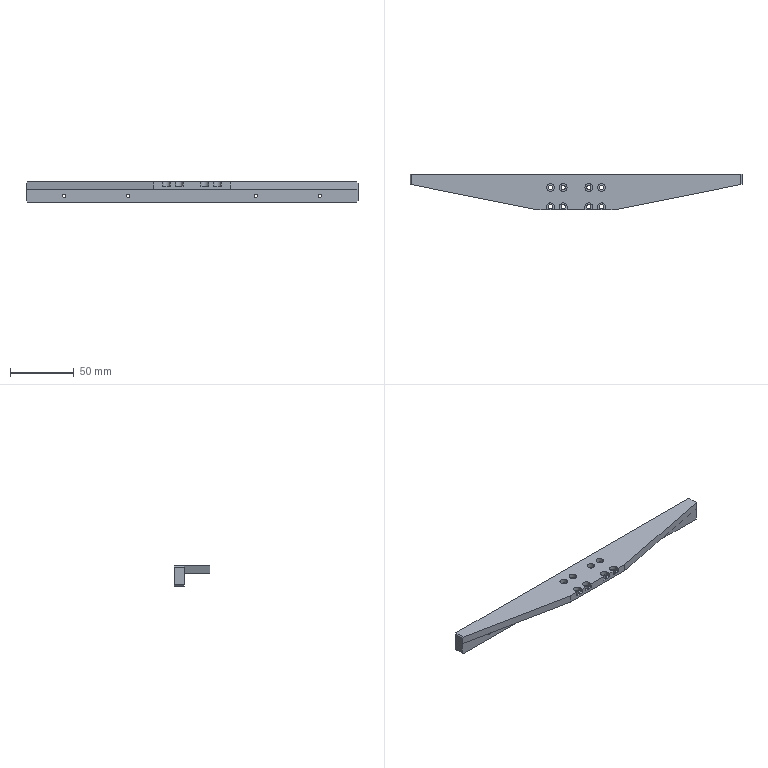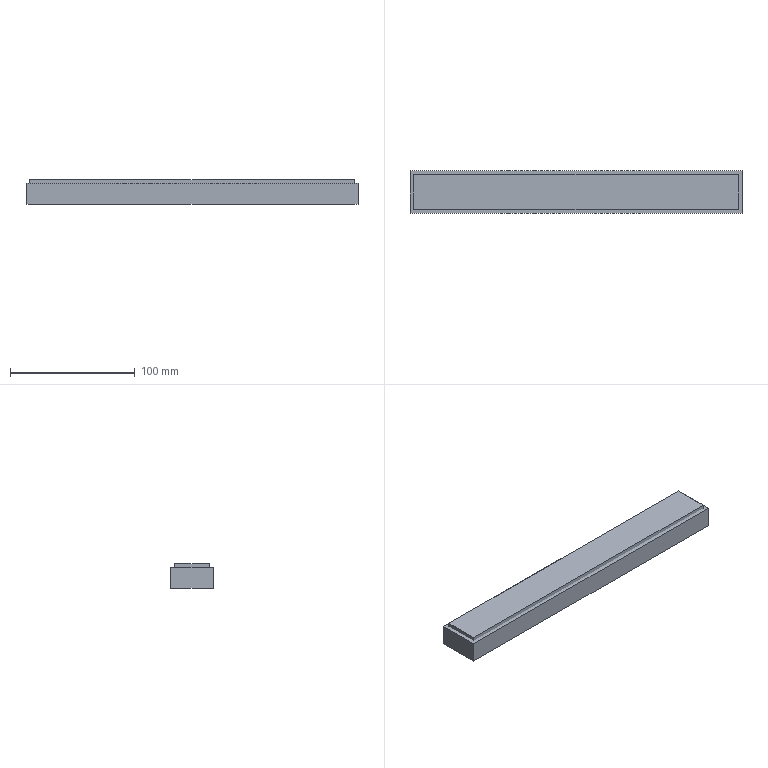CAM job | NX | 3+2 milling, drilling | part box 260 x 28 x 16 mm | stock box 266 x 34 x 20 mm
Tools:
number,name,description,diameter,corner_radius,flute_length,length,flutes
19,D80,Milling Tool-5 Parameters,80.0,0.0,50.0,75.0,2
15,D10,Milling Tool-5 Parameters,10.0,0.0,50.0,75.0,2
14,D10JING,Milling Tool-5 Parameters,10.0,0.0,50.0,75.0,2
1,D6A45,Milling Tool-5 Parameters,6.0,0.0,50.0,75.0,2
16,3.4ZT,Drilling Tool,3.4,0.0,35.0,50.0,2
11,D4,Milling Tool-5 Parameters,4.0,0.0,50.0,75.0,2
2,2.5ZT,Drilling Tool,2.5,0.0,35.0,50.0,2
3,D3,Milling Tool-5 Parameters,3.0,0.0,50.0,75.0,2
Operations:
program,operation,operation_type,tool,method,geometry_group,spindle_rpm,surface_speed,feed_per_tooth,feed_cut,feed_plunge,cut_length_mm,path_length_mm,cut_time_min,machine_time_min
1,FLOOR_WALL,VolumeBased25DMillingOperation,D80,METHOD,A,6500.0,1633.0,0.1154,1500.0,100.0,358.0,412.0,0.2387,0.2441
1,CAVITY_MILL,CavityMilling,D10,METHOD,A,9500.0,298.0,0.1842,3500.0,1000.0,32708.204,33169.87,9.46,9.506
1,ZLEVEL_PROFILE,ZLevelMilling,D10JING,METHOD,A,9500.0,298.0,0.0789,1500.0,1000.0,579.715,668.715,0.3878,0.3967
1,FLOOR_WALL_1,VolumeBased25DMillingOperation,D10JING,METHOD,A,9500.0,298.0,0.0658,1250.0,100.0,1166.837,1581.927,0.9335,0.975
1,PLANAR_MILL,PlanarMilling,D6A45,METHOD,A,9500.0,179.0,0.0658,1250.0,100.0,548.194,607.194,0.4386,0.4445
1,PLANAR_MILL_COPY,PlanarMilling,D6A45,METHOD,A,9500.0,179.0,0.0658,1250.0,100.0,244.439,323.438,0.1956,0.2035
2,FLOOR_WALL_COPY,VolumeBased25DMillingOperation,D80,METHOD,B,6500.0,1633.0,0.1154,1500.0,100.0,1408.0,2650.001,0.9387,1.063
2,DRILLING,Operation,D6A45,METHOD,B,9500.0,179.0,0.0132,250.0,0.0,32.0,237.579,0.128,0.1486
2,DRILLING_COPY,Operation,3.4ZT,METHOD,B,2000.0,21.0,0.0375,150.0,0.0,92.172,357.923,0.6145,0.6411
2,HOLE_MILLING,CylinderMilling,D4,METHOD,B,9500.0,179.0,0.0329,1250.0,100.0,318.184,609.784,0.2545,0.2837
2,ZLEVEL_PROFILE_1,ZLevelMilling,D4,METHOD,B,9500.0,119.0,0.1053,2000.0,100.0,544.149,907.163,0.2721,0.3084
2,PLANAR_MILL_COPY_1,PlanarMilling,D6A45,METHOD,B,9500.0,179.0,0.0658,1250.0,100.0,657.566,997.813,0.5261,0.5601
3,DRILLING_COPY_1,Operation,D6A45,METHOD,C,9500.0,179.0,0.0132,250.0,0.0,44.0,427.731,0.176,0.2144
3,DRILLING_COPY_COPY,Operation,2.5ZT,METHOD,C,2000.0,21.0,0.0375,150.0,0.0,109.26,550.806,0.7284,0.7726
3,HOLE_MILLING_1,CylinderMilling,D3,METHOD,C,9500.0,89.0,0.0526,1000.0,100.0,117.222,473.221,0.1172,0.1528
3,PLANAR_MILL_COPY_1_COPY,PlanarMilling,D6A45,METHOD,C,9500.0,179.0,0.0658,1250.0,100.0,640.635,1608.612,0.5125,0.6093
3,刀补,CylinderMilling,D3,METHOD,C,9500.0,89.0,0.0526,1000.0,100.0,30.964,386.964,0.031,0.0666